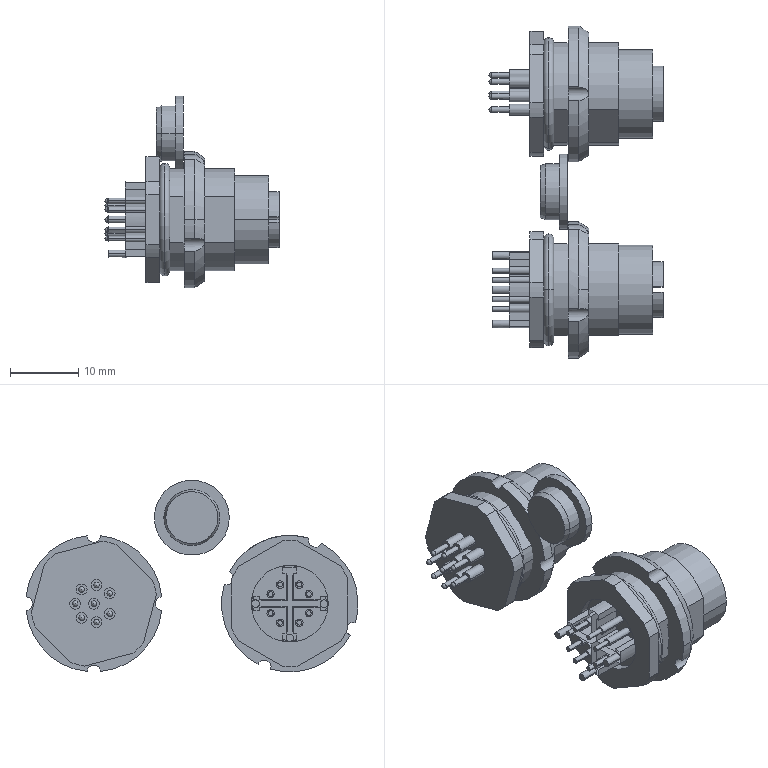Part | NX | features BREP 7 | 7 solids | 323 faces | box 25.5 x 48.65 x 28.1 mm | volume 6463 mm3 | cylinder 173 | plane 122 | cone 12 | sphere 8 | torus 8 | commonest cylinder face diameters 0.7 x48 1.1 x22 0.8 x16 1.6 x16 18.5 x12 2 x11